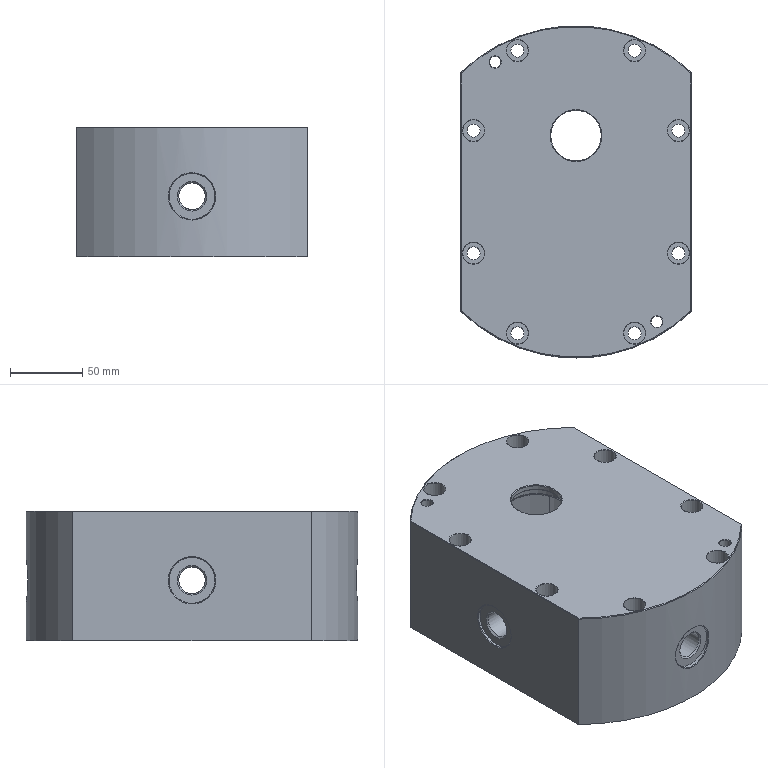NC program | NX | posted with a generic post | part box 160 x 230 x 90 mm
Whole program:
N10 G17 G21 G94 G90
(FLOOR_WALL , TOOL : D50)
N12 T02 M6
N14 G54
N16 G17 G0 G90 X-46.915 Y54.997 B0. C0. S1200 M3
N18 G43 Z30. H2
N20 Z2.651
N22 G94 G1 Z-0.349 F1000.
N24 X-43.915
N26 X43.915 F2000.
N28 Y24.998
N30 X-43.915
N32 Y-5.001
N34 X43.915
N36 Y-35.
N38 X-43.915
N40 X-46.915
N42 Z2.651
N44 G0 Z30.
N46 X-50.601 Y54.997
N48 Z2.302
N50 G1 Z-0.698 F1000.
N52 X-47.601
N54 X47.601 F2000.
N56 Y24.998
N58 X-47.601
N60 Y-5.001
N62 X47.601
N64 Y-35.
N66 X-47.601
N68 X-50.601
N70 Z2.302
N72 G0 Z30.
N74 X-53.452 Y54.997
N76 Z1.953
N78 G1 Z-1.047 F1000.
N80 X-50.452
N82 X50.452 F2000.
N84 Y24.998
N86 X-50.452
N88 Y-5.001
N90 X50.452
N92 Y-35.
N94 X-50.452
N96 X-53.452
N98 Z1.953
N100 G0 Z30.
N102 X-55.849 Y54.997
N104 Z1.604
N106 G1 Z-1.396 F1000.
N108 X-52.849
N110 X52.849 F2000.
N112 Y24.998
N114 X-52.849
N116 Y-5.001
N118 X52.849
N120 Y-35.
N122 X-52.849
N124 X-55.849
N126 Z1.604
N128 G0 Z30.
N130 X-57.905 Y54.997
N132 Z1.255
N134 G1 Z-1.745 F1000.
N136 X-54.905
N138 X54.905 F2000.
N140 Y24.998
N142 X-54.905
N144 Y-5.001
N146 X54.905
N148 Y-35.
N150 X-54.905
N152 X-57.905
N154 Z1.255
N156 G0 Z30.
N158 X-59.807 Y54.997
N160 Z0.906
N162 G1 Z-2.094 F1000.
N164 X-56.807
N166 X56.807 F2000.
N168 Y24.998
N170 X-56.807
N172 Y-5.001
N174 X56.807
N176 Y-35.
N178 X-56.807
N180 X-59.807
N182 Z0.906
N184 G0 Z30.
N186 X-61.554 Y54.997
N188 Z0.557
N190 G1 Z-2.443 F1000.
N192 X-58.554
N194 X58.554 F2000.
N196 Y24.998
N198 X-58.554
N200 Y-5.001
N202 X58.554
N204 Y-35.
N206 X-58.554
N208 X-61.554
N210 Z0.557
N212 G0 Z30.
N214 X-63.145 Y54.997
N216 Z0.208
N218 G1 Z-2.792 F1000.
N220 X-60.145
N222 X60.145 F2000.
N224 Y24.998
N226 X-60.145
N228 Y-5.001
N230 X60.145
N232 Y-35.
N234 X-60.145
N236 X-63.145
N238 Z0.208
N240 G0 Z30.
N242 X-64.681 Y54.997
N244 Z-0.141
N246 G1 Z-3.141 F1000.
N248 X-61.681
N250 X61.681 F2000.
N252 Y24.998
N254 X-61.681
N256 Y-5.001
N258 X61.681
N260 Y-35.
N262 X-61.681
N264 X-64.681
N266 Z-0.141
N268 G0 Z30.
N270 X-66.079 Y54.997
N272 Z-0.49
N274 G1 Z-3.49 F1000.
N276 X-63.079
N278 X63.079 F2000.
N280 Y24.998
N282 X-63.079
N284 Y-5.001
N286 X63.079
N288 Y-35.
N290 X-63.079
N292 X-66.079
N294 Z-0.49
N296 G0 Z30.
N298 X-67.447 Y54.997
N300 Z-0.839
N302 G1 Z-3.839 F1000.
N304 X-64.447
N306 X64.447 F2000.
N308 Y24.998
N310 X-64.447
N312 Y-5.001
N314 X64.447
N316 Y-35.
N318 X-64.447
N320 X-67.447
N322 Z-0.839
N324 G0 Z30.
N326 X-68.723 Y54.997
N328 Z-1.188
N330 G1 Z-4.188 F1000.
N332 X-65.723
N334 X65.723 F2000.
N336 Y24.998
N338 X-65.723
N340 Y-5.001
N342 X65.723
N344 Y-35.
N346 X-65.723
N348 X-68.723
N350 Z-1.188
N352 G0 Z30.
N354 X-69.955 Y54.997
N356 Z-1.537
N358 G1 Z-4.537 F1000.
N360 X-66.955
N362 X66.955 F2000.
N364 Y24.998
N366 X-66.955
N368 Y-5.001
N370 X66.955
N372 Y-35.
N374 X-66.955
N376 X-69.955
N378 Z-1.537
N380 G0 Z30.
N382 X-71.151 Y54.997
N384 Z-1.886
N386 G1 Z-4.886 F1000.
N388 X-68.151
N390 X68.151 F2000.
N392 Y24.998
N394 X-68.151
N396 Y-5.001
N398 X68.151
N400 Y-35.
N402 X-68.151
N404 X-71.151
N406 Z-1.886
N408 G0 Z30.
N410 X-72.27 Y54.997
N412 Z-2.235
N414 G1 Z-5.235 F1000.
N416 X-69.27
N418 X69.27 F2000.
N420 Y24.998
N422 X-69.27
N424 Y-5.001
N426 X69.27
N428 Y-35.
N430 X-69.27
N432 X-72.27
N434 Z-2.235
N436 G0 Z30.
N438 X-73.389 Y54.997
N440 Z-2.584
N442 G1 Z-5.584 F1000.
N444 X-70.389
N446 X70.389 F2000.
N448 Y24.998
N450 X-70.389
N452 Y-5.001
N454 X70.389
N456 Y-35.
N458 X-70.389
N460 X-73.389
N462 Z-2.584
N464 G0 Z30.
N466 X-74.437 Y54.997
N468 Z-2.933
N470 G1 Z-5.933 F1000.
N472 X-71.437
N474 X71.437 F2000.
N476 Y24.998
N478 X-71.437
N480 Y-5.001
N482 X71.437
N484 Y-35.
N486 X-71.437
N488 X-74.437
N490 Z-2.933
N492 G0 Z30.
N494 X-75.461 Y54.997
N496 Z-3.282
N498 G1 Z-6.282 F1000.
N500 X-72.461
N502 X72.461 F2000.
N504 Y24.998
N506 X-72.461
N508 Y-5.001
N510 X72.461
N512 Y-35.
N514 X-72.461
N516 X-75.461
N518 Z-3.282
N520 G0 Z30.
N522 X-76.478 Y54.997
N524 Z-3.631
N526 G1 Z-6.631 F1000.
N528 X-73.478
N530 X73.478 F2000.
N532 Y24.998
N534 X-73.478
N536 Y-5.001
N538 X73.478
N540 Y-35.
N542 X-73.478
N544 X-76.478
N546 Z-3.631
N548 G0 Z30.
N550 X-77.431 Y54.997
N552 Z-3.98
N554 G1 Z-6.98 F1000.
N556 X-74.431
N558 X74.431 F2000.
N560 Y24.998
N562 X-74.431
N564 Y-5.001
N566 X74.431
N568 Y-35.
N570 X-74.431
N572 X-77.431
N574 Z-3.98
N576 G0 Z30.
N578 X-78.372 Y54.997
N580 Z-4.329
N582 G1 Z-7.329 F1000.
N584 X-75.372
N586 X75.372 F2000.
N588 Y24.998
N590 X-75.372
N592 Y-5.001
N594 X75.372
N596 Y-35.
N598 X-75.372
N600 X-78.372
N602 Z-4.329
N604 G0 Z30.
N606 X-79.311 Y54.997
N608 Z-4.678
N610 G1 Z-7.678 F1000.
N612 X-76.311
N614 X76.311 F2000.
N616 Y24.998
N618 X-76.311
N620 Y-5.001
N622 X76.311
N624 Y-35.
N626 X-76.311
N628 X-79.311
N630 Z-4.678
N632 G0 Z30.
N634 X-80.189 Y54.997
N636 Z-5.027
N638 G1 Z-8.027 F1000.
N640 X-77.189
N642 X77.189 F2000.
N644 Y24.998
N646 X-77.189
N648 Y-5.001
N650 X77.189
N652 Y-35.
N654 X-77.189
N656 X-80.189
N658 Z-5.027
N660 G0 Z30.
N662 X-81.06 Y54.997
N664 Z-5.376
N666 G1 Z-8.376 F1000.
N668 X-78.06
N670 X78.06 F2000.
N672 Y24.998
N674 X-78.06
N676 Y-5.001
N678 X78.06
N680 Y-35.
N682 X-78.06
N684 X-81.06
N686 Z-5.376
N688 G0 Z30.
N690 X-81.931 Y54.997
N692 Z-5.725
N694 G1 Z-8.725 F1000.
N696 X-78.931
N698 X78.931 F2000.
N700 Y24.998
N702 X-78.931
N704 Y-5.001
N706 X78.931
N708 Y-35.
N710 X-78.931
N712 X-81.931
N714 Z-5.725
N716 G0 Z30.
N718 X-82.757 Y54.997
N720 Z-6.074
N722 G1 Z-9.074 F1000.
N724 X-79.757
N726 X79.757 F2000.
N728 Y24.998
N730 X-79.757
N732 Y-5.001
N734 X79.757
N736 Y-35.
N738 X-79.757
N740 X-82.757
N742 Z-6.074
N744 G0 Z30.
N746 X-83.566 Y54.997
N748 Z-6.423
N750 G1 Z-9.423 F1000.
N752 X-80.566
N754 X80.566 F2000.
N756 Y24.998
N758 X-80.566
N760 Y-5.001
N762 X80.566
N764 Y-35.
N766 X-80.565
N768 X-83.565
N770 Z-6.423
N772 G0 Z30.
N774 X-84.374 Y54.997
N776 Z-6.772
N778 G1 Z-9.772 F1000.
N780 X-81.374
N782 X81.374 F2000.
N784 Y24.998
N786 X-81.374
N788 Y-5.001
N790 X81.374
N792 Y-35.
N794 X-81.374
N796 X-84.374
N798 Z-6.772
N800 G0 Z30.
N802 X-85.168 Y54.997
N804 Z-7.121
N806 G1 Z-10.121 F1000.
N808 X-82.168
N810 X82.168 F2000.
N812 Y24.998
N814 X-82.168
N816 Y-5.001
N818 X82.168
N820 Y-35.
N822 X-82.168
N824 X-85.168
N826 Z-7.121
N828 G0 Z30.
N830 X-85.921 Y54.997
N832 Z-7.47
N834 G1 Z-10.47 F1000.
N836 X-82.921
N838 X82.921 F2000.
N840 Y24.998
N842 X-82.921
N844 Y-5.001
N846 X82.921
N848 Y-35.
N850 X-82.921
N852 X-85.921
N854 Z-7.47
N856 G0 Z30.
N858 X-86.675 Y54.997
N860 Z-7.819
N862 G1 Z-10.819 F1000.
N864 X-83.675
N866 X83.675 F2000.
N868 Y24.998
N870 X-83.675
N872 Y-5.001
N874 X83.675
N876 Y-35.
N878 X-83.675
N880 X-86.675
N882 Z-7.819
N884 G0 Z30.
N886 X-87.428 Y54.997
N888 Z-8.168
N890 G1 Z-11.168 F1000.
N892 X-84.428
N894 X84.428 F2000.
N896 Y24.998
N898 X-84.428
N900 Y-5.001
N902 X84.428
N904 Y-35.
N906 X-84.428
N908 X-87.428
N910 Z-8.168
N912 G0 Z30.
N914 X-88.15 Y54.997
N916 Z-8.517
N918 G1 Z-11.517 F1000.
N920 X-85.15
N922 X85.15 F2000.
N924 Y24.998
N926 X-85.15
N928 Y-5.001
N930 X85.15
N932 Y-35.
N934 X-85.15
N936 X-88.15
N938 Z-8.517
N940 G0 Z30.
N942 X-88.855 Y54.997
N944 Z-8.866
N946 G1 Z-11.866 F1000.
N948 X-85.855
N950 X85.855 F2000.
N952 Y24.998
N954 X-85.855
N956 Y-5.001
N958 X85.855
N960 Y-35.
N962 X-85.855
N964 X-88.855
N966 Z-8.866
N968 G0 Z30.
N970 X-89.559 Y54.997
N972 Z-9.215
N974 G1 Z-12.215 F1000.
N976 X-86.559
N978 X86.559 F2000.
N980 Y24.998
N982 X-86.559
N984 Y-5.001
N986 X86.559
N988 Y-35.
N990 X-86.559
N992 X-89.559
N994 Z-9.215
N996 G0 Z30.
N998 X-90.261 Y54.997
N1000 Z-9.564
N1002 G1 Z-12.564 F1000.
N1004 X-87.261
N1006 X87.261 F2000.
N1008 Y24.998
N1010 X-87.261
N1012 Y-5.001
N1014 X87.261
N1016 Y-35.
N1018 X-87.261
N1020 X-90.261
N1022 Z-9.564
N1024 G0 Z30.
N1026 X-90.932 Y54.997
N1028 Z-9.913
N1030 G1 Z-12.913 F1000.
N1032 X-87.932
N1034 X87.932 F2000.
N1036 Y24.998
N1038 X-87.932
N1040 Y-5.001
N1042 X87.932
N1044 Y-35.
N1046 X-87.932
N1048 X-90.932
N1050 Z-9.913
N1052 G0 Z30.
N1054 X-91.593 Y54.997
N1056 Z-10.262
N1058 G1 Z-13.262 F1000.
N1060 X-88.593
N1062 X88.593 F2000.
N1064 Y24.998
N1066 X-88.593
N1068 Y-5.001
N1070 X88.593
N1072 Y-35.
N1074 X-88.593
N1076 X-91.593
N1078 Z-10.262
N1080 G0 Z30.
N1082 X-92.253 Y54.997
N1084 Z-10.611
N1086 G1 Z-13.611 F1000.
N1088 X-89.253
N1090 X89.253 F2000.
N1092 Y24.998
N1094 X-89.253
N1096 Y-5.001
N1098 X89.253
N1100 Y-35.
N1102 X-89.253
N1104 X-92.253
N1106 Z-10.611
N1108 G0 Z30.
N1110 X-92.91 Y54.997
N1112 Z-10.96
N1114 G1 Z-13.96 F1000.
N1116 X-89.91
N1118 X89.91 F2000.
N1120 Y24.998
N1122 X-89.91
N1124 Y-5.001
N1126 X89.91
N1128 Y-35.
N1130 X-89.91
N1132 X-92.91
N1134 Z-10.96
N1136 G0 Z30.
N1138 X-93.543 Y54.997
N1140 Z-11.309
N1142 G1 Z-14.309 F1000.
N1144 X-90.543
N1146 X90.543 F2000.
N1148 Y24.998
N1150 X-90.543
N1152 Y-5.001
N1154 X90.543
N1156 Y-35.
N1158 X-90.543
N1160 X-93.543
N1162 Z-11.309
N1164 G0 Z30.
N1166 X-94.163 Y54.997
N1168 Z-11.658
N1170 G1 Z-14.658 F1000.
N1172 X-91.163
N1174 X91.163 F2000.
N1176 Y24.998
N1178 X-91.163
N1180 Y-5.001
N1182 X91.163
N1184 Y-35.
N1186 X-91.163
N1188 X-94.163
N1190 Z-11.658
N1192 G0 Z30.
N1194 X-94.783 Y54.997
N1196 Z-12.007
N1198 G1 Z-15.007 F1000.
N1200 X-91.783
N1202 X91.783 F2000.
N1204 Y24.998
N1206 X-91.783
N1208 Y-5.001
N1210 X91.783
N1212 Y-35.
N1214 X-91.783
N1216 X-94.783
N1218 Z-12.007
N1220 G0 Z30.
N1222 X-95.403 Y54.997
N1224 Z-12.356
N1226 G1 Z-15.356 F1000.
N1228 X-92.403
N1230 X92.403 F2000.
N1232 Y24.998
N1234 X-92.403
N1236 Y-5.001
N1238 X92.403
N1240 Y-35.
N1242 X-92.403
N1244 X-95.403
N1246 Z-12.356
N1248 G0 Z30.
N1250 X-96.005 Y54.997
N1252 Z-12.705
N1254 G1 Z-15.705 F1000.
N1256 X-93.005
N1258 X93.005 F2000.
N1260 Y24.998
N1262 X-93.005
N1264 Y-5.001
N1266 X93.005
N1268 Y-35.
N1270 X-93.005
N1272 X-96.005
N1274 Z-12.705
N1276 G0 Z30.
N1278 X-96.589 Y54.997
N1280 Z-13.054
N1282 G1 Z-16.054 F1000.
N1284 X-93.589
N1286 X93.589 F2000.
N1288 Y24.998
N1290 X-93.589
N1292 Y-5.001
N1294 X93.589
N1296 Y-35.
N1298 X-93.589
N1300 X-96.589
N1302 Z-13.054
N1304 G0 Z30.
N1306 X-97.173 Y54.997
N1308 Z-13.403
N1310 G1 Z-16.403 F1000.
N1312 X-94.173
N1314 X94.173 F2000.
N1316 Y24.998
N1318 X-94.173
N1320 Y-5.001
N1322 X94.173
N1324 Y-35.
N1326 X-94.173
N1328 X-97.173
N1330 Z-13.403
N1332 G0 Z30.
N1334 X-97.756 Y54.997
N1336 Z-13.752
N1338 G1 Z-16.752 F1000.
N1340 X-94.756
N1342 X94.756 F2000.
N1344 Y24.998
N1346 X-94.756
N1348 Y-5.001
N1350 X94.756
N1352 Y-35.
N1354 X-94.756
N1356 X-97.756
N1358 Z-13.752
N1360 G0 Z30.
N1362 X-98.337 Y54.997
N1364 Z-14.101
N1366 G1 Z-17.101 F1000.
N1368 X-95.337
N1370 X95.337 F2000.
N1372 Y24.998
N1374 X-95.337
N1376 Y-5.001
N1378 X95.337
N1380 Y-35.
N1382 X-95.337
N1384 X-98.337
N1386 Z-14.101
N1388 G0 Z30.
N1390 X-98.889 Y54.997
N1392 Z-14.45
N1394 G1 Z-17.45 F1000.
N1396 X-95.889
N1398 X95.889 F2000.
N1400 Y24.998
N1402 X-95.889
N1404 Y-5.001
N1406 X95.889
N1408 Y-35.
N1410 X-95.889
N1412 X-98.889
N1414 Z-14.45
N1416 G0 Z30.
N1418 X-99.439 Y54.997
N1420 Z-14.799
N1422 G1 Z-17.799 F1000.
N1424 X-96.439
N1426 X96.439 F2000.
N1428 Y24.998
N1430 X-96.439
N1432 Y-5.001
N1434 X96.439
N1436 Y-35.
N1438 X-96.439
N1440 X-99.439
N1442 Z-14.799
N1444 G0 Z30.
N1446 X-99.989 Y54.997
N1448 Z-15.148
N1450 G1 Z-18.148 F1000.
N1452 X-96.989
N1454 X96.989 F2000.
N1456 Y24.998
N1458 X-96.989
N1460 Y-5.001
N1462 X96.989
N1464 Y-35.
N1466 X-96.989
N1468 X-99.989
N1470 Z-15.148
N1472 G0 Z30.
N1474 X-100.539 Y54.997
N1476 Z-15.497
N1478 G1 Z-18.497 F1000.
N1480 X-97.539
N1482 X97.539 F2000.
N1484 Y24.998
N1486 X-97.539
N1488 Y-5.001
N1490 X97.539
N1492 Y-35.
N1494 X-97.539
N1496 X-100.539
N1498 Z-15.497
N1500 G0 Z30.
N1502 X-101.077 Y54.997
N1504 Z-15.846
N1506 G1 Z-18.846 F1000.
N1508 X-98.077
N1510 X98.077 F2000.
N1512 Y24.998
N1514 X-98.077
N1516 Y-5.001
N1518 X98.077
N1520 Y-35.
N1522 X-98.077
N1524 X-101.077
N1526 Z-15.846
N1528 G0 Z30.
N1530 X-101.597 Y54.997
N1532 Z-16.195
N1534 G1 Z-19.195 F1000.
N1536 X-98.597
N1538 X98.597 F2000.
N1540 Y24.998
N1542 X-98.597
N1544 Y-5.001
N1546 X98.597
N1548 Y-35.
N1550 X-98.597
N1552 X-101.597
N1554 Z-16.195
N1556 G0 Z30.
N1558 X-102.116 Y54.997
N1560 Z-16.544
N1562 G1 Z-19.544 F1000.
N1564 X-99.116
N1566 X99.116 F2000.
N1568 Y24.998
N1570 X-99.116
N1572 Y-5.001
N1574 X99.116
N1576 Y-35.
N1578 X-99.116
N1580 X-102.116
N1582 Z-16.544
N1584 G0 Z30.
N1586 X-102.636 Y54.997
N1588 Z-16.893
N1590 G1 Z-19.893 F1000.
N1592 X-99.636
N1594 X99.636 F2000.
N1596 Y24.998
N1598 X-99.636
N1600 Y-5.001
N1602 X99.636
N1604 Y-35.
N1606 X-99.636
N1608 X-102.636
N1610 Z-16.893
N1612 G0 Z30.
N1614 X-103.155 Y54.997
N1616 Z-17.242
N1618 G1 Z-20.242 F1000.
N1620 X-100.155
N1622 X100.155 F2000.
N1624 Y24.998
N1626 X-100.155
N1628 Y-5.001
N1630 X100.155
N1632 Y-35.
N1634 X-100.155
N1636 X-103.155
N1638 Z-17.242
N1640 G0 Z30.
N1642 X-103.658 Y54.997
N1644 Z-17.591
N1646 G1 Z-20.591 F1000.
N1648 X-100.658
N1650 X100.658 F2000.
N1652 Y24.998
N1654 X-100.658
N1656 Y-5.001
N1658 X100.658
N1660 Y-35.
N1662 X-100.658
N1664 X-103.658
N1666 Z-17.591
N1668 G0 Z30.
N1670 X-104.15 Y54.997
N1672 Z-17.94
N1674 G1 Z-20.94 F1000.
N1676 X-101.15
N1678 X101.15 F2000.
N1680 Y24.998
N1682 X-101.15
N1684 Y-5.001
N1686 X101.15
N1688 Y-35.
N1690 X-101.15
N1692 X-104.15
N1694 Z-17.94
N1696 G0 Z30.
N1698 X-104.641 Y54.997
N1700 Z-18.289
N1702 G1 Z-21.289 F1000.
N1704 X-101.641
N1706 X101.641 F2000.
N1708 Y24.998
N1710 X-101.641
N1712 Y-5.001
N1714 X101.641
N1716 Y-35.
N1718 X-101.641
N1720 X-104.641
N1722 Z-18.289
N1724 G0 Z30.
N1726 X-105.132 Y54.997
N1728 Z-18.638
N1730 G1 Z-21.638 F1000.
N1732 X-102.132
N1734 X102.132 F2000.
N1736 Y24.998
N1738 X-102.132
N1740 Y-5.001
N1742 X102.132
N1744 Y-35.
N1746 X-102.132
N1748 X-105.132
N1750 Z-18.638
N1752 G0 Z30.
N1754 X-105.623 Y54.997
N1756 Z-18.987
N1758 G1 Z-21.987 F1000.
N1760 X-102.623
N1762 X102.623 F2000.
N1764 Y24.998
N1766 X-102.623
N1768 Y-5.001
N1770 X102.623
N1772 Y-35.
N1774 X-102.623
N1776 X-105.623
N1778 Z-18.987
N1780 G0 Z30.
N1782 X-106.099 Y54.997
N1784 Z-19.336
N1786 G1 Z-22.336 F1000.
N1788 X-103.099
N1790 X103.099 F2000.
N1792 Y24.998
N1794 X-103.099
N1796 Y-5.001
N1798 X103.099
N1800 Y-35.
N1802 X-103.099
N1804 X-106.099
N1806 Z-19.336
N1808 G0 Z30.
N1810 X-106.564 Y54.997
N1812 Z-19.685
N1814 G1 Z-22.685 F1000.
N1816 X-103.564
N1818 X103.564 F2000.
N1820 Y24.998
N1822 X-103.564
N1824 Y-5.001
N1826 X103.564
N1828 Y-35.
N1830 X-103.564
N1832 X-106.564
N1834 Z-19.685
N1836 G0 Z30.
N1838 X-107.029 Y54.997
N1840 Z-20.034
N1842 G1 Z-23.034 F1000.
N1844 X-104.029
N1846 X104.029 F2000.
N1848 Y24.998
N1850 X-104.029
N1852 Y-5.001
N1854 X104.029
N1856 Y-35.
N1858 X-104.029
N1860 X-107.029
N1862 Z-20.034
N1864 G0 Z30.
N1866 X-107.494 Y54.997
N1868 Z-20.383
N1870 G1 Z-23.383 F1000.
N1872 X-104.494
N1874 X104.494 F2000.
N1876 Y24.998
N1878 X-104.494
N1880 Y-5.001
N1882 X104.494
N1884 Y-35.
N1886 X-104.494
N1888 X-107.494
N1890 Z-20.383
N1892 G0 Z30.
N1894 X-107.958 Y54.997
N1896 Z-20.732
N1898 G1 Z-23.732 F1000.
N1900 X-104.958
N1902 X104.958 F2000.
N1904 Y24.998
N1906 X-104.958
N1908 Y-5.001
N1910 X104.958
N1912 Y-35.
N1914 X-104.958
N1916 X-107.958
N1918 Z-20.732
N1920 G0 Z30.
N1922 X-108.414 Y54.997
N1924 Z-21.081
N1926 G1 Z-24.081 F1000.
N1928 X-105.414
N1930 X105.414 F2000.
N1932 Y24.998
N1934 X-105.414
N1936 Y-5.001
N1938 X105.414
N1940 Y-35.
N1942 X-105.414
N1944 X-108.414
N1946 Z-21.081
N1948 G0 Z30.
N1950 X-108.855 Y54.997
N1952 Z-21.43
N1954 G1 Z-24.43 F1000.
N1956 X-105.855
N1958 X105.855 F2000.
N1960 Y24.998
N1962 X-105.855
N1964 Y-5.001
N1966 X105.855
N1968 Y-35.
N1970 X-105.855
N1972 X-108.855
N1974 Z-21.43
N1976 G0 Z30.
N1978 X-109.295 Y54.997
N1980 Z-21.779
N1982 G1 Z-24.779 F1000.
N1984 X-106.295
N1986 X106.295 F2000.
N1988 Y24.998
N1990 X-106.295
N1992 Y-5.001
N1994 X106.295
N1996 Y-35.
N1998 X-106.295
N2000 X-109.295
N2002 Z-21.779
N2004 G0 Z30.
N2006 X-109.735 Y54.997
N2008 Z-22.128
N2010 G1 Z-25.128 F1000.
N2012 X-106.735
N2014 X106.735 F2000.
N2016 Y24.998
N2018 X-106.735
N2020 Y-5.001
N2022 X106.735
N2024 Y-35.
N2026 X-106.735
N2028 X-109.735
N2030 Z-22.128
N2032 G0 Z30.
N2034 X-110.175 Y54.997
N2036 Z-22.477
N2038 G1 Z-25.477 F1000.
N2040 X-107.175
N2042 X107.175 F2000.
N2044 Y24.998
N2046 X-107.175
N2048 Y-5.001
N2050 X107.175
N2052 Y-35.
N2054 X-107.175
N2056 X-110.175
N2058 Z-22.477
N2060 G0 Z30.
N2062 X-110.612 Y54.997
N2064 Z-22.826
N2066 G1 Z-25.826 F1000.
N2068 X-107.612
N2070 X107.612 F2000.
N2072 Y24.998
N2074 X-107.612
N2076 Y-5.001
N2078 X107.612
N2080 Y-35.
N2082 X-107.612
N2084 X-110.612
N2086 Z-22.826
N2088 G0 Z30.
N2090 X-111.033 Y54.997
N2092 Z-23.175
N2094 G1 Z-26.175 F1000.
N2096 X-108.033
N2098 X108.033 F2000.
N2100 Y24.998
N2102 X-108.033
N2104 Y-5.001
N2106 X108.033
N2108 Y-35.
N2110 X-108.033
N2112 X-111.033
N2114 Z-23.175
N2116 G0 Z30.
N2118 X-111.45 Y54.997
N2120 Z-23.524
N2122 G1 Z-26.524 F1000.
N2124 X-108.45
N2126 X108.45 F2000.
N2128 Y24.998
N2130 X-108.45
N2132 Y-5.001
N2134 X108.45
N2136 Y-35.
N2138 X-108.45
N2140 X-111.45
N2142 Z-23.524
N2144 G0 Z30.
N2146 X-111.867 Y54.997
N2148 Z-23.873
N2150 G1 Z-26.873 F1000.
N2152 X-108.867
N2154 X108.867 F2000.
N2156 Y24.998
N2158 X-108.867
N2160 Y-5.001
N2162 X108.867
N2164 Y-35.
N2166 X-108.867
N2168 X-111.867
N2170 Z-23.873
N2172 G0 Z30.
N2174 X-112.284 Y54.997
N2176 Z-24.222
N2178 G1 Z-27.222 F1000.
N2180 X-109.284
N2182 X109.284 F2000.
N2184 Y24.998
N2186 X-109.284
N2188 Y-5.001
N2190 X109.284
N2192 Y-35.
N2194 X-109.284
N2196 X-112.284
N2198 Z-24.222
N2200 G0 Z30.
N2202 X-112.701 Y54.997
N2204 Z-24.571
N2206 G1 Z-27.571 F1000.
N2208 X-109.701
N2210 X109.701 F2000.
N2212 Y24.998
N2214 X-109.701
N2216 Y-5.001
N2218 X109.701
N2220 Y-35.
N2222 X-109.701
N2224 X-112.701
N2226 Z-24.571
N2228 G0 Z30.
N2230 X-113.11 Y54.997
N2232 Z-24.92
N2234 G1 Z-27.92 F1000.
N2236 X-110.11
N2238 X110.11 F2000.
N2240 Y24.998
N2242 X-110.11
N2244 Y-5.001
N2246 X110.11
N2248 Y-35.
N2250 X-110.11
N2252 X-113.11
N2254 Z-24.92
N2256 G0 Z30.
N2258 X-113.505 Y54.997
N2260 Z-25.269
N2262 G1 Z-28.269 F1000.
N2264 X-110.505
N2266 X110.505 F2000.
N2268 Y24.998
N2270 X-110.505
N2272 Y-5.001
N2274 X110.505
N2276 Y-35.
N2278 X-110.505
N2280 X-113.505
N2282 Z-25.269
N2284 G0 Z30.
N2286 X-113.901 Y54.997
N2288 Z-25.618
N2290 G1 Z-28.618 F1000.
N2292 X-110.901
N2294 X110.901 F2000.
N2296 Y24.998
N2298 X-110.901
N2300 Y-5.001
N2302 X110.901
N2304 Y-35.
N2306 X-110.901
N2308 X-113.901
N2310 Z-25.618
N2312 G0 Z30.
N2314 X-114.296 Y54.997
N2316 Z-25.967
N2318 G1 Z-28.967 F1000.
N2320 X-111.296
N2322 X111.296 F2000.
N2324 Y24.998
N2326 X-111.296
N2328 Y-5.001
N2330 X111.296
N2332 Y-35.
N2334 X-111.296
N2336 X-114.296
N2338 Z-25.967
N2340 G0 Z30.
N2342 X-114.692 Y54.997
N2344 Z-26.316
N2346 G1 Z-29.316 F1000.
N2348 X-111.692
N2350 X111.692 F2000.
N2352 Y24.998
N2354 X-111.692
N2356 Y-5.001
N2358 X111.692
N2360 Y-35.
N2362 X-111.692
N2364 X-114.692
N2366 Z-26.316
N2368 G0 Z30.
N2370 X-115.085 Y54.997
N2372 Z-26.665
N2374 G1 Z-29.665 F1000.
N2376 X-112.085
N2378 X112.085 F2000.
N2380 Y24.998
N2382 X-112.085
N2384 Y-5.001
N2386 X112.085
N2388 Y-35.
N2390 X-112.085
N2392 X-115.085
N2394 Z-26.665
N2396 G0 Z30.
N2398 X-115.469 Y54.997
N2400 Z-27.014
N2402 G1 Z-30.014 F1000.
N2404 X-112.469
N2406 X112.469 F2000.
N2408 Y24.998
N2410 X-112.469
N2412 Y-5.001
N2414 X112.469
N2416 Y-35.
N2418 X-112.469
N2420 X-115.469
N2422 Z-27.014
N2424 G0 Z30.
N2426 X-115.844 Y54.997
N2428 Z-27.363
N2430 G1 Z-30.363 F1000.
N2432 X-112.844
N2434 X112.844 F2000.
N2436 Y24.998
N2438 X-112.844
N2440 Y-5.001
N2442 X112.844
N2444 Y-35.
N2446 X-112.844
N2448 X-115.844
N2450 Z-27.363
N2452 G0 Z30.
N2454 X-116.219 Y54.997
N2456 Z-27.712
N2458 G1 Z-30.712 F1000.
N2460 X-113.219
N2462 X113.219 F2000.
N2464 Y24.998
N2466 X-113.219
N2468 Y-5.001
N2470 X113.219
N2472 Y-35.
N2474 X-113.219
N2476 X-116.219
N2478 Z-27.712
N2480 G0 Z30.
N2482 X-116.595 Y54.997
N2484 Z-28.061
N2486 G1 Z-31.061 F1000.
N2488 X-113.595
N2490 X113.595 F2000.
N2492 Y24.998
N2494 X-113.595
N2496 Y-5.001
N2498 X113.595
N2500 Y-35.
N2502 X-113.595
N2504 X-116.595
N2506 Z-28.061
N2508 G0 Z30.
N2510 X-116.97 Y54.997
N2512 Z-28.41
N2514 G1 Z-31.41 F1000.
N2516 X-113.97
N2518 X113.97 F2000.
N2520 Y24.998
N2522 X-113.97
N2524 Y-5.001
N2526 X113.97
N2528 Y-35.
N2530 X-113.97
N2532 X-116.97
N2534 Z-28.41
N2536 G0 Z30.
N2538 X-117.343 Y54.997
N2540 Z-28.759
N2542 G1 Z-31.759 F1000.
N2544 X-114.343
N2546 X114.343 F2000.
N2548 Y24.998
N2550 X-114.343
N2552 Y-5.001
N2554 X114.343
N2556 Y-35.
N2558 X-114.343
N2560 X-117.343
N2562 Z-28.759
N2564 G0 Z30.
N2566 X-117.705 Y54.997
N2568 Z-29.108
N2570 G1 Z-32.108 F1000.
N2572 X-114.705
N2574 X114.705 F2000.
N2576 Y24.998
N2578 X-114.705
N2580 Y-5.001
N2582 X114.705
N2584 Y-35.
N2586 X-114.705
N2588 X-117.705
N2590 Z-29.108
N2592 G0 Z30.
N2594 X-118.061 Y54.997
N2596 Z-29.457
N2598 G1 Z-32.457 F1000.
N2600 X-115.061
N2602 X115.061 F2000.
N2604 Y24.998
N2606 X-115.061
N2608 Y-5.001
N2610 X115.061
N2612 Y-35.
N2614 X-115.061
N2616 X-118.061
N2618 Z-29.457
N2620 G0 Z30.
N2622 X-118.417 Y54.997
N2624 Z-29.806
N2626 G1 Z-32.806 F1000.
N2628 X-115.417
N2630 X115.417 F2000.
N2632 Y24.998
N2634 X-115.417
N2636 Y-5.001
N2638 X115.417
N2640 Y-35.
N2642 X-115.417
N2644 X-118.417
N2646 Z-29.806
N2648 G0 Z30.
N2650 X-118.773 Y54.997
N2652 Z-30.155
N2654 G1 Z-33.155 F1000.
N2656 X-115.773
N2658 X115.773 F2000.
N2660 Y24.998
N2662 X-115.773
N2664 Y-5.001
N2666 X115.773
N2668 Y-35.
N2670 X-115.773
N2672 X-118.773
N2674 Z-30.155
N2676 G0 Z30.
N2678 X-119.129 Y54.997
N2680 Z-30.504
N2682 G1 Z-33.504 F1000.
N2684 X-116.129
N2686 X116.129 F2000.
N2688 Y24.998
N2690 X-116.129
N2692 Y-5.001
N2694 X116.129
N2696 Y-35.
N2698 X-116.129
N2700 X-119.129
N2702 Z-30.504
N2704 G0 Z30.
N2706 X-119.484 Y54.997
N2708 Z-30.853
N2710 G1 Z-33.853 F1000.
N2712 X-116.484
N2714 X116.484 F2000.
N2716 Y24.998
N2718 X-116.484
N2720 Y-5.001
N2722 X116.484
N2724 Y-35.
N2726 X-116.484
N2728 X-119.484
N2730 Z-30.853
N2732 G0 Z30.
N2734 X-119.828 Y54.997
N2736 Z-31.202
N2738 G1 Z-34.202 F1000.
N2740 X-116.828
N2742 X116.828 F2000.
N2744 Y24.998
N2746 X-116.828
N2748 Y-5.001
N2750 X116.828
N2752 Y-35.
N2754 X-116.828
N2756 X-119.828
N2758 Z-31.202
N2760 G0 Z30.
N2762 X-120.165 Y54.997
N2764 Z-31.551
N2766 G1 Z-34.551 F1000.
N2768 X-117.165
N2770 X117.165 F2000.
N2772 Y24.998
N2774 X-117.165
N2776 Y-5.001
N2778 X117.165
N2780 Y-35.
N2782 X-117.165
N2784 X-120.165
N2786 Z-31.551
N2788 G0 Z30.
N2790 X-120.5 Y54.997
N2792 Z-31.9
N2794 G1 Z-34.9 F1000.
N2796 X-117.5
N2798 X117.5 F2000.
N2800 Y24.998
N2802 X-117.5
N2804 Y-5.001
N2806 X117.5
N2808 Y-35.
N2810 X-117.5
N2812 X-120.5
N2814 Z-31.9
N2816 G0 Z30.
(FLOOR_WALL_COPY , TOOL : D50)
N2818 X-120.597 Y54.997 S2500
N2820 Z-32.
N2822 G1 Z-35. F1000.
N2824 X-117.597
N2826 X117.597
N2828 Y24.998
N2830 X-117.597
N2832 Y-5.001
N2834 X117.597
N2836 Y-35.
N2838 X-117.597
N2840 X-120.597
N2842 Z-32.
N2844 G0 Z30.
N2846 M5
(HOLE_MILLING , TOOL : D10)
N2848 T10 M6
N2850 G54
N2852 G17 G0 G90 X0. Y-3. B0. C0. S3000 M3
N2854 G43 Z30. H10
N2856 Z-34.5
N2858 G94 G3 X1.817 Y-4.817 R1.817 F2200.
N2860 X3.633 Y-3. R1.817
N2862 X3.633 Y-3. Z-34.72 I-3.633 J0.
N2864 X3.633 Y-3. Z-34.94 I-3.633 J0.
N2866 X3.633 Y-3. Z-35.16 I-3.633 J0.
N2868 X3.633 Y-3. Z-35.38 I-3.633 J0.
N2870 X3.633 Y-3. Z-35.6 I-3.633 J0.
N2872 X3.633 Y-3. Z-35.82 I-3.633 J0.
N2874 X3.633 Y-3. Z-36.04 I-3.633 J0.
N2876 X3.633 Y-3. Z-36.26 I-3.633 J0.
N2878 X3.633 Y-3. Z-36.48 I-3.633 J0.
N2880 X3.633 Y-3. Z-36.7 I-3.633 J0.
N2882 X3.633 Y-3. Z-36.92 I-3.633 J0.
N2884 X-2.379 Y-0.254 Z-37. R3.633
N2886 X-2.746 Y-5.379 R3.633
N2888 X-2.379 Y-0.254 R-3.633
N2890 X-2.563 Y-2.817 R1.817
N2892 X0. Y-3. R1.817
N2894 G0 Z-34.5
N2896 G3 X3.633 Y-6.633 R3.633
N2898 X7.267 Y-3. R3.633
N2900 X7.267 Y-3. Z-34.72 I-7.267 J0.
N2902 X7.267 Y-3. Z-34.94 I-7.267 J0.
N2904 X7.267 Y-3. Z-35.16 I-7.267 J0.
N2906 X7.267 Y-3. Z-35.38 I-7.267 J0.
N2908 X7.267 Y-3. Z-35.6 I-7.267 J0.
N2910 X7.267 Y-3. Z-35.82 I-7.267 J0.
N2912 X7.267 Y-3. Z-36.04 I-7.267 J0.
N2914 X7.267 Y-3. Z-36.26 I-7.267 J0.
N2916 X7.267 Y-3. Z-36.48 I-7.267 J0.
N2918 X7.267 Y-3. Z-36.7 I-7.267 J0.
N2920 X7.267 Y-3. Z-36.92 I-7.267 J0.
N2922 X-4.759 Y2.492 Z-37. R7.267
N2924 X-5.492 Y-7.759 R7.267
N2926 X-4.759 Y2.492 R-7.267
N2928 X-5.125 Y-2.633 R3.633
N2930 X0. Y-3. R3.633
N2932 G0 Z-34.5
N2934 G3 X5.45 Y-8.45 R5.45
N2936 X10.9 Y-3. R5.45
N2938 X10.9 Y-3. Z-34.72 I-10.9 J0.
N2940 X10.9 Y-3. Z-34.94 I-10.9 J0.
N2942 X10.9 Y-3. Z-35.16 I-10.9 J0.
N2944 X10.9 Y-3. Z-35.38 I-10.9 J0.
N2946 X10.9 Y-3. Z-35.6 I-10.9 J0.
N2948 X10.9 Y-3. Z-35.82 I-10.9 J0.
N2950 X10.9 Y-3. Z-36.04 I-10.9 J0.
N2952 X10.9 Y-3. Z-36.26 I-10.9 J0.
N2954 X10.9 Y-3. Z-36.48 I-10.9 J0.
N2956 X10.9 Y-3. Z-36.7 I-10.9 J0.
N2958 X10.9 Y-3. Z-36.92 I-10.9 J0.
N2960 X-7.138 Y5.238 Z-37. R10.9
N2962 X-8.238 Y-10.138 R10.9
N2964 X-7.138 Y5.238 R-10.9
N2966 X-7.688 Y-2.45 R5.45
N2968 X0. Y-3. R5.45
N2970 G0 Z30.
(HOLE_MILLING_COPY , TOOL : D10)
N2972 Z-36.5
N2974 G3 X2.075 Y-5.075 R2.075
N2976 X4.15 Y-3. R2.075
N2978 X4.15 Y-3. Z-36.72 I-4.15 J0.
N2980 X4.15 Y-3. Z-36.94 I-4.15 J0.
N2982 X4.15 Y-3. Z-37.16 I-4.15 J0.
N2984 X4.15 Y-3. Z-37.38 I-4.15 J0.
N2986 X4.15 Y-3. Z-37.6 I-4.15 J0.
N2988 X4.15 Y-3. Z-37.82 I-4.15 J0.
N2990 X4.15 Y-3. Z-38.04 I-4.15 J0.
N2992 X4.15 Y-3. Z-38.26 I-4.15 J0.
N2994 X4.15 Y-3. Z-38.48 I-4.15 J0.
N2996 X4.15 Y-3. Z-38.7 I-4.15 J0.
N2998 X4.15 Y-3. Z-38.92 I-4.15 J0.
N3000 X4.15 Y-3. Z-39.14 I-4.15 J0.
N3002 X4.15 Y-3. Z-39.36 I-4.15 J0.
N3004 X4.15 Y-3. Z-39.58 I-4.15 J0.
N3006 X4.15 Y-3. Z-39.8 I-4.15 J0.
N3008 X4.15 Y-3. Z-40.02 I-4.15 J0.
N3010 X4.15 Y-3. Z-40.24 I-4.15 J0.
N3012 X4.15 Y-3. Z-40.46 I-4.15 J0.
N3014 X4.15 Y-3. Z-40.68 I-4.15 J0.
N3016 X4.15 Y-3. Z-40.9 I-4.15 J0.
N3018 X4.15 Y-3. Z-41.12 I-4.15 J0.
N3020 X4.15 Y-3. Z-41.34 I-4.15 J0.
N3022 X4.15 Y-3. Z-41.56 I-4.15 J0.
N3024 X4.15 Y-3. Z-41.78 I-4.15 J0.
N3026 X4.15 Y-3. Z-42. I-4.15 J0.
N3028 X4.15 Y-3. Z-42.22 I-4.15 J0.
N3030 X4.15 Y-3. Z-42.44 I-4.15 J0.
N3032 X4.15 Y-3. Z-42.66 I-4.15 J0.
N3034 X4.15 Y-3. Z-42.88 I-4.15 J0.
N3036 X4.15 Y-3. Z-43.1 I-4.15 J0.
N3038 X4.15 Y-3. Z-43.32 I-4.15 J0.
N3040 X4.15 Y-3. Z-43.54 I-4.15 J0.
N3042 X4.15 Y-3. Z-43.76 I-4.15 J0.
N3044 X4.15 Y-3. Z-43.98 I-4.15 J0.
N3046 X4.15 Y-3. Z-44.2 I-4.15 J0.
N3048 X4.15 Y-3. Z-44.42 I-4.15 J0.
N3050 X4.15 Y-3. Z-44.64 I-4.15 J0.
N3052 X4.15 Y-3. Z-44.86 I-4.15 J0.
N3054 X4.15 Y-3. Z-45.08 I-4.15 J0.
N3056 X4.15 Y-3. Z-45.3 I-4.15 J0.
N3058 X4.15 Y-3. Z-45.52 I-4.15 J0.
N3060 X4.15 Y-3. Z-45.74 I-4.15 J0.
N3062 X4.15 Y-3. Z-45.96 I-4.15 J0.
N3064 X4.15 Y-3. Z-46.18 I-4.15 J0.
N3066 X4.15 Y-3. Z-46.4 I-4.15 J0.
N3068 X4.15 Y-3. Z-46.62 I-4.15 J0.
N3070 X4.15 Y-3. Z-46.84 I-4.15 J0.
N3072 X4.15 Y-3. Z-47.06 I-4.15 J0.
N3074 X4.15 Y-3. Z-47.28 I-4.15 J0.
N3076 X4.15 Y-3. Z-47.5 I-4.15 J0.
N3078 X4.15 Y-3. Z-47.72 I-4.15 J0.
N3080 X4.15 Y-3. Z-47.94 I-4.15 J0.
N3082 X4.15 Y-3. Z-48.16 I-4.15 J0.
N3084 X4.15 Y-3. Z-48.38 I-4.15 J0.
N3086 X4.15 Y-3. Z-48.6 I-4.15 J0.
N3088 X4.15 Y-3. Z-48.82 I-4.15 J0.
N3090 X4.15 Y-3. Z-49.04 I-4.15 J0.
N3092 X4.15 Y-3. Z-49.26 I-4.15 J0.
N3094 X4.15 Y-3. Z-49.48 I-4.15 J0.
N3096 X4.15 Y-3. Z-49.7 I-4.15 J0.
N3098 X4.15 Y-3. Z-49.92 I-4.15 J0.
N3100 X4.15 Y-3. Z-50.14 I-4.15 J0.
N3102 X4.15 Y-3. Z-50.36 I-4.15 J0.
N3104 X4.15 Y-3. Z-50.58 I-4.15 J0.
N3106 X4.15 Y-3. Z-50.8 I-4.15 J0.
N3108 X4.15 Y-3. Z-51.02 I-4.15 J0.
N3110 X4.15 Y-3. Z-51.24 I-4.15 J0.
N3112 X4.15 Y-3. Z-51.46 I-4.15 J0.
N3114 X4.15 Y-3. Z-51.68 I-4.15 J0.
N3116 X4.15 Y-3. Z-51.9 I-4.15 J0.
N3118 X4.15 Y-3. Z-52.12 I-4.15 J0.
N3120 X4.15 Y-3. Z-52.34 I-4.15 J0.
N3122 X4.15 Y-3. Z-52.56 I-4.15 J0.
N3124 X4.15 Y-3. Z-52.78 I-4.15 J0.
N3126 X4.15 Y-3. Z-53. I-4.15 J0.
N3128 X4.15 Y-3. Z-53.22 I-4.15 J0.
N3130 X4.15 Y-3. Z-53.44 I-4.15 J0.
N3132 X4.15 Y-3. Z-53.66 I-4.15 J0.
N3134 X4.15 Y-3. Z-53.88 I-4.15 J0.
N3136 X4.15 Y-3. Z-54.1 I-4.15 J0.
N3138 X4.15 Y-3. Z-54.32 I-4.15 J0.
N3140 X4.15 Y-3. Z-54.54 I-4.15 J0.
N3142 X4.15 Y-3. Z-54.76 I-4.15 J0.
N3144 X4.15 Y-3. Z-54.98 I-4.15 J0.
N3146 X4.15 Y-3. Z-55.2 I-4.15 J0.
N3148 X4.15 Y-3. Z-55.42 I-4.15 J0.
N3150 X4.15 Y-3. Z-55.64 I-4.15 J0.
N3152 X4.15 Y-3. Z-55.86 I-4.15 J0.
N3154 X4.15 Y-3. Z-56.08 I-4.15 J0.
N3156 X4.15 Y-3. Z-56.3 I-4.15 J0.
N3158 X4.15 Y-3. Z-56.52 I-4.15 J0.
N3160 X4.15 Y-3. Z-56.74 I-4.15 J0.
N3162 X4.15 Y-3. Z-56.96 I-4.15 J0.
N3164 X1.724 Y0.775 Z-57. R4.15
N3166 X-3.775 Y-1.276 R4.15
N3168 X1.724 Y0.775 R-4.15
N3170 X-1.026 Y-0.251 R2.075
N3172 X0. Y-3. R2.075
N3174 G0 Z30.
N3176 M5
(HOLE_MILLING_COPY_1 , TOOL : D10JING)
N3178 T11 M6
N3180 G54
N3182 G17 G0 G90 X0. Y-3. B0. C0. S5000 M3
N3184 G43 Z30. H11
N3186 Z-37.
N3188 G94 G1 X7.486 Y-5.524 F1000.
N3190 G3 X11. Y-3. R2.663
N3192 X0. Y8. R11.
N3194 X11. Y-3. R-11.
N3196 X7.486 Y-0.476 R2.663
N3198 G1 X0. Y-3.
N3200 G0 Z30.
(HOLE_MILLING_COPY_1_COPY , TOOL : D10JING)
N3202 Z-57.
N3204 G1 X0.58 Y-3.993
N3206 G3 X4.25 Y-3. R1.969
N3208 X0. Y1.25 R4.25
N3210 X4.25 Y-3. R-4.25
N3212 X0.58 Y-2.007 R1.969
N3214 G1 X0. Y-3.
N3216 G0 Z30.
N3218 M5
(PLANAR_MILL , TOOL : D6A45)
N3220 T07 M6
N3222 G54
N3224 G17 G0 G90 X-83.875 Y46.7 B0. C0. S7500 M3
N3226 G43 Z30. H7
N3228 Z-33.
N3230 G94 G1 Z-36. F1250.
N3232 X-83.168 Y45.857
N3234 G3 X-82.401 Y45.5 R1.
N3236 G1 X82.401
N3238 G3 X83.168 Y45.857 R1.
N3240 G1 X83.875 Y46.7
N3242 Z-33.
N3244 G0 Z30.
N3246 X84.087 Y-46.7
N3248 Z-33.
N3250 G1 Z-36.
N3252 X83.38 Y-45.857
N3254 G3 X82.614 Y-45.5 R1.
N3256 G1 X-82.614
N3258 G3 X-83.38 Y-45.857 R1.
N3260 G1 X-84.087 Y-46.7
N3262 Z-33.
N3264 G0 Z30.
N3266 X1.543 Y11.216
N3268 Z-33.
N3270 G1 Z-36.
N3272 X0.766 Y12.143
N3274 G3 X0. Y12.5 R1.
N3276 X-15.5 Y-3. R15.5
N3278 X0. Y12.5 R-15.5
N3280 X-0.766 Y12.143 R1.
N3282 G1 X-1.543 Y11.216
N3284 Z-33.
N3286 G0 Z30.
(PLANAR_MILL_COPY , TOOL : D6A45)
N3288 X1.634 Y3.858
N3290 Z-35.5
N3292 G1 Z-38.5
N3294 X0.766 Y4.893
N3296 G3 X0. Y5.25 R1.
N3298 X-8.25 Y-3. R8.25
N3300 X0. Y5.25 R-8.25
N3302 X-0.766 Y4.893 R1.
N3304 G1 X-1.634 Y3.858
N3306 Z-35.5
N3308 G0 Z30.
N3310 M5
N3312 M2